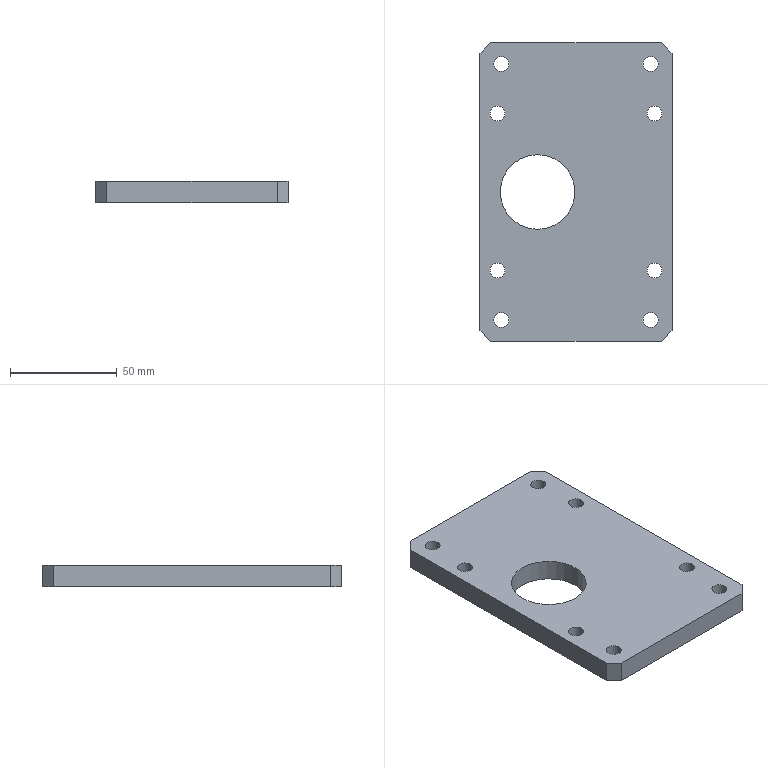Part | NX | features 5003_202_Mounting plate 2 | 1 solid | 19 faces | box 90 x 140 x 10 mm | volume 112800 mm3 | plane 10 | cylinder 9 | commonest cylinder face diameters 7 x8 35 x1
STEP:
#1=CARTESIAN_POINT('',(136.525,-252.,-325.));
#2=VERTEX_POINT('',#1);
#3=CARTESIAN_POINT('',(216.525,-252.,-325.));
#4=VERTEX_POINT('',#3);
#5=CARTESIAN_POINT('',(158.525,-252.,-325.));
#6=DIRECTION('',(1.,0.,0.));
#7=VECTOR('',#6,1000.);
#8=LINE('',#5,#7);
#9=EDGE_CURVE('',#2,#4,#8,.T.);
#10=ORIENTED_EDGE('',*,*,#9,.T.);
#11=CARTESIAN_POINT('',(216.525,-252.,-335.));
#12=VERTEX_POINT('',#11);
#13=CARTESIAN_POINT('',(216.525,-252.,-335.));
#14=DIRECTION('',(0.,0.,-1.));
#15=VECTOR('',#14,1000.);
#16=LINE('',#13,#15);
#17=EDGE_CURVE('',#4,#12,#16,.T.);
#18=ORIENTED_EDGE('',*,*,#17,.T.);
#19=CARTESIAN_POINT('',(136.525,-252.,-335.));
#20=VERTEX_POINT('',#19);
#21=CARTESIAN_POINT('',(158.525,-252.,-335.));
#22=DIRECTION('',(1.,0.,0.));
#23=VECTOR('',#22,1000.);
#24=LINE('',#21,#23);
#25=EDGE_CURVE('',#20,#12,#24,.T.);
#26=ORIENTED_EDGE('',*,*,#25,.F.);
#27=CARTESIAN_POINT('',(136.525,-252.,-325.));
#28=DIRECTION('',(0.,0.,1.));
#29=VECTOR('',#28,1000.);
#30=LINE('',#27,#29);
#31=EDGE_CURVE('',#20,#2,#30,.T.);
#32=ORIENTED_EDGE('',*,*,#31,.T.);
#33=EDGE_LOOP('',(#10,#18,#26,#32));
#34=FACE_BOUND('',#33,.T.);
#35=CARTESIAN_POINT('',(158.525,-252.,-325.));
#36=DIRECTION('',(0.,1.,0.));
#37=DIRECTION('',(0.,0.,-1.));
#38=AXIS2_PLACEMENT_3D('',#35,#36,#37);
#39=PLANE('',#38);
#40=ADVANCED_FACE('',(#34),#39,.T.);
#41=CARTESIAN_POINT('',(131.525,-387.,-325.));
#42=VERTEX_POINT('',#41);
#43=CARTESIAN_POINT('',(131.525,-257.,-325.));
#44=VERTEX_POINT('',#43);
#45=CARTESIAN_POINT('',(131.525,-322.,-325.));
#46=DIRECTION('',(0.,1.,0.));
#47=VECTOR('',#46,1000.);
#48=LINE('',#45,#47);
#49=EDGE_CURVE('',#42,#44,#48,.T.);
#50=ORIENTED_EDGE('',*,*,#49,.T.);
#51=CARTESIAN_POINT('',(131.525,-257.,-335.));
#52=VERTEX_POINT('',#51);
#53=CARTESIAN_POINT('',(131.525,-257.,-325.));
#54=DIRECTION('',(0.,0.,-1.));
#55=VECTOR('',#54,1000.);
#56=LINE('',#53,#55);
#57=EDGE_CURVE('',#44,#52,#56,.T.);
#58=ORIENTED_EDGE('',*,*,#57,.T.);
#59=CARTESIAN_POINT('',(131.525,-387.,-335.));
#60=VERTEX_POINT('',#59);
#61=CARTESIAN_POINT('',(131.525,-322.,-335.));
#62=DIRECTION('',(0.,1.,0.));
#63=VECTOR('',#62,1000.);
#64=LINE('',#61,#63);
#65=EDGE_CURVE('',#60,#52,#64,.T.);
#66=ORIENTED_EDGE('',*,*,#65,.F.);
#67=CARTESIAN_POINT('',(131.525,-387.,-325.));
#68=DIRECTION('',(0.,0.,1.));
#69=VECTOR('',#68,1000.);
#70=LINE('',#67,#69);
#71=EDGE_CURVE('',#60,#42,#70,.T.);
#72=ORIENTED_EDGE('',*,*,#71,.T.);
#73=EDGE_LOOP('',(#50,#58,#66,#72));
#74=FACE_BOUND('',#73,.T.);
#75=CARTESIAN_POINT('',(131.525,-322.,-325.));
#76=DIRECTION('',(-1.,0.,0.));
#77=DIRECTION('',(0.,0.,1.));
#78=AXIS2_PLACEMENT_3D('',#75,#76,#77);
#79=PLANE('',#78);
#80=ADVANCED_FACE('',(#74),#79,.T.);
#81=CARTESIAN_POINT('',(136.525,-392.,-325.));
#82=VERTEX_POINT('',#81);
#83=CARTESIAN_POINT('',(216.525,-392.,-325.));
#84=VERTEX_POINT('',#83);
#85=CARTESIAN_POINT('',(158.525,-392.,-325.));
#86=DIRECTION('',(1.,0.,0.));
#87=VECTOR('',#86,1000.);
#88=LINE('',#85,#87);
#89=EDGE_CURVE('',#82,#84,#88,.T.);
#90=ORIENTED_EDGE('',*,*,#89,.F.);
#91=CARTESIAN_POINT('',(136.525,-392.,-335.));
#92=VERTEX_POINT('',#91);
#93=CARTESIAN_POINT('',(136.525,-392.,-335.));
#94=DIRECTION('',(0.,0.,-1.));
#95=VECTOR('',#94,1000.);
#96=LINE('',#93,#95);
#97=EDGE_CURVE('',#82,#92,#96,.T.);
#98=ORIENTED_EDGE('',*,*,#97,.T.);
#99=CARTESIAN_POINT('',(216.525,-392.,-335.));
#100=VERTEX_POINT('',#99);
#101=CARTESIAN_POINT('',(158.525,-392.,-335.));
#102=DIRECTION('',(1.,0.,0.));
#103=VECTOR('',#102,1000.);
#104=LINE('',#101,#103);
#105=EDGE_CURVE('',#92,#100,#104,.T.);
#106=ORIENTED_EDGE('',*,*,#105,.T.);
#107=CARTESIAN_POINT('',(216.525,-392.,-325.));
#108=DIRECTION('',(0.,0.,1.));
#109=VECTOR('',#108,1000.);
#110=LINE('',#107,#109);
#111=EDGE_CURVE('',#100,#84,#110,.T.);
#112=ORIENTED_EDGE('',*,*,#111,.T.);
#113=EDGE_LOOP('',(#90,#98,#106,#112));
#114=FACE_BOUND('',#113,.T.);
#115=CARTESIAN_POINT('',(158.525,-392.,-325.));
#116=DIRECTION('',(0.,1.,0.));
#117=DIRECTION('',(-1.,0.,0.));
#118=AXIS2_PLACEMENT_3D('',#115,#116,#117);
#119=PLANE('',#118);
#120=ADVANCED_FACE('',(#114),#119,.F.);
#121=CARTESIAN_POINT('',(211.525,-258.5,-325.));
#122=VERTEX_POINT('',#121);
#123=CARTESIAN_POINT('',(211.525,-262.,-325.));
#124=DIRECTION('',(0.,0.,1.));
#125=DIRECTION('',(0.,1.,0.));
#126=AXIS2_PLACEMENT_3D('',#123,#124,#125);
#127=CIRCLE('',#126,3.5);
#128=EDGE_CURVE('',#122,#122,#127,.F.);
#129=ORIENTED_EDGE('',*,*,#128,.F.);
#130=EDGE_LOOP('',(#129));
#131=FACE_BOUND('',#130,.T.);
#132=CARTESIAN_POINT('',(211.525,-258.5,-335.));
#133=VERTEX_POINT('',#132);
#134=CARTESIAN_POINT('',(211.525,-262.,-335.));
#135=DIRECTION('',(0.,0.,1.));
#136=DIRECTION('',(0.,1.,0.));
#137=AXIS2_PLACEMENT_3D('',#134,#135,#136);
#138=CIRCLE('',#137,3.5);
#139=EDGE_CURVE('',#133,#133,#138,.F.);
#140=ORIENTED_EDGE('',*,*,#139,.T.);
#141=EDGE_LOOP('',(#140));
#142=FACE_BOUND('',#141,.T.);
#143=CARTESIAN_POINT('',(211.525,-262.,-325.));
#144=DIRECTION('',(0.,0.,-1.));
#145=DIRECTION('',(0.,-1.,0.));
#146=AXIS2_PLACEMENT_3D('',#143,#144,#145);
#147=CYLINDRICAL_SURFACE('',#146,3.5);
#148=ADVANCED_FACE('',(#131,#142),#147,.F.);
#149=CARTESIAN_POINT('',(158.525,-304.5,-325.));
#150=VERTEX_POINT('',#149);
#151=CARTESIAN_POINT('',(158.525,-322.,-325.));
#152=DIRECTION('',(0.,0.,1.));
#153=DIRECTION('',(0.,1.,0.));
#154=AXIS2_PLACEMENT_3D('',#151,#152,#153);
#155=CIRCLE('',#154,17.5);
#156=EDGE_CURVE('',#150,#150,#155,.T.);
#157=ORIENTED_EDGE('',*,*,#156,.T.);
#158=EDGE_LOOP('',(#157));
#159=FACE_BOUND('',#158,.T.);
#160=CARTESIAN_POINT('',(158.525,-304.5,-335.));
#161=VERTEX_POINT('',#160);
#162=CARTESIAN_POINT('',(158.525,-322.,-335.));
#163=DIRECTION('',(0.,0.,1.));
#164=DIRECTION('',(0.,1.,0.));
#165=AXIS2_PLACEMENT_3D('',#162,#163,#164);
#166=CIRCLE('',#165,17.5);
#167=EDGE_CURVE('',#161,#161,#166,.T.);
#168=ORIENTED_EDGE('',*,*,#167,.F.);
#169=EDGE_LOOP('',(#168));
#170=FACE_BOUND('',#169,.T.);
#171=CARTESIAN_POINT('',(158.525,-322.,-325.));
#172=DIRECTION('',(0.,0.,-1.));
#173=DIRECTION('',(0.,-1.,0.));
#174=AXIS2_PLACEMENT_3D('',#171,#172,#173);
#175=CYLINDRICAL_SURFACE('',#174,17.5);
#176=ADVANCED_FACE('',(#159,#170),#175,.F.);
#177=CARTESIAN_POINT('',(141.525,-378.5,-325.));
#178=VERTEX_POINT('',#177);
#179=CARTESIAN_POINT('',(141.525,-382.,-325.));
#180=DIRECTION('',(0.,0.,1.));
#181=DIRECTION('',(0.,1.,0.));
#182=AXIS2_PLACEMENT_3D('',#179,#180,#181);
#183=CIRCLE('',#182,3.5);
#184=EDGE_CURVE('',#178,#178,#183,.T.);
#185=ORIENTED_EDGE('',*,*,#184,.T.);
#186=EDGE_LOOP('',(#185));
#187=FACE_BOUND('',#186,.T.);
#188=CARTESIAN_POINT('',(141.525,-378.5,-335.));
#189=VERTEX_POINT('',#188);
#190=CARTESIAN_POINT('',(141.525,-382.,-335.));
#191=DIRECTION('',(0.,0.,1.));
#192=DIRECTION('',(0.,1.,0.));
#193=AXIS2_PLACEMENT_3D('',#190,#191,#192);
#194=CIRCLE('',#193,3.5);
#195=EDGE_CURVE('',#189,#189,#194,.T.);
#196=ORIENTED_EDGE('',*,*,#195,.F.);
#197=EDGE_LOOP('',(#196));
#198=FACE_BOUND('',#197,.T.);
#199=CARTESIAN_POINT('',(141.525,-382.,-325.));
#200=DIRECTION('',(0.,0.,-1.));
#201=DIRECTION('',(0.,-1.,0.));
#202=AXIS2_PLACEMENT_3D('',#199,#200,#201);
#203=CYLINDRICAL_SURFACE('',#202,3.5);
#204=ADVANCED_FACE('',(#187,#198),#203,.F.);
#205=CARTESIAN_POINT('',(139.745,-355.28,-325.));
#206=VERTEX_POINT('',#205);
#207=CARTESIAN_POINT('',(139.745,-358.78,-325.));
#208=DIRECTION('',(0.,0.,1.));
#209=DIRECTION('',(0.,1.,0.));
#210=AXIS2_PLACEMENT_3D('',#207,#208,#209);
#211=CIRCLE('',#210,3.5);
#212=EDGE_CURVE('',#206,#206,#211,.T.);
#213=ORIENTED_EDGE('',*,*,#212,.T.);
#214=EDGE_LOOP('',(#213));
#215=FACE_BOUND('',#214,.T.);
#216=CARTESIAN_POINT('',(139.745,-355.28,-335.));
#217=VERTEX_POINT('',#216);
#218=CARTESIAN_POINT('',(139.745,-358.78,-335.));
#219=DIRECTION('',(0.,0.,1.));
#220=DIRECTION('',(0.,1.,0.));
#221=AXIS2_PLACEMENT_3D('',#218,#219,#220);
#222=CIRCLE('',#221,3.5);
#223=EDGE_CURVE('',#217,#217,#222,.T.);
#224=ORIENTED_EDGE('',*,*,#223,.F.);
#225=EDGE_LOOP('',(#224));
#226=FACE_BOUND('',#225,.T.);
#227=CARTESIAN_POINT('',(139.745,-358.78,-325.));
#228=DIRECTION('',(0.,0.,-1.));
#229=DIRECTION('',(0.,-1.,0.));
#230=AXIS2_PLACEMENT_3D('',#227,#228,#229);
#231=CYLINDRICAL_SURFACE('',#230,3.5);
#232=ADVANCED_FACE('',(#215,#226),#231,.F.);
#233=CARTESIAN_POINT('',(211.525,-378.5,-325.));
#234=VERTEX_POINT('',#233);
#235=CARTESIAN_POINT('',(211.525,-382.,-325.));
#236=DIRECTION('',(0.,0.,1.));
#237=DIRECTION('',(0.,1.,0.));
#238=AXIS2_PLACEMENT_3D('',#235,#236,#237);
#239=CIRCLE('',#238,3.5);
#240=EDGE_CURVE('',#234,#234,#239,.T.);
#241=ORIENTED_EDGE('',*,*,#240,.T.);
#242=EDGE_LOOP('',(#241));
#243=FACE_BOUND('',#242,.T.);
#244=CARTESIAN_POINT('',(211.525,-378.5,-335.));
#245=VERTEX_POINT('',#244);
#246=CARTESIAN_POINT('',(211.525,-382.,-335.));
#247=DIRECTION('',(0.,0.,1.));
#248=DIRECTION('',(0.,1.,0.));
#249=AXIS2_PLACEMENT_3D('',#246,#247,#248);
#250=CIRCLE('',#249,3.5);
#251=EDGE_CURVE('',#245,#245,#250,.T.);
#252=ORIENTED_EDGE('',*,*,#251,.F.);
#253=EDGE_LOOP('',(#252));
#254=FACE_BOUND('',#253,.T.);
#255=CARTESIAN_POINT('',(211.525,-382.,-325.));
#256=DIRECTION('',(0.,0.,-1.));
#257=DIRECTION('',(0.,-1.,0.));
#258=AXIS2_PLACEMENT_3D('',#255,#256,#257);
#259=CYLINDRICAL_SURFACE('',#258,3.5);
#260=ADVANCED_FACE('',(#243,#254),#259,.F.);
#261=CARTESIAN_POINT('',(213.305,-355.28,-325.));
#262=VERTEX_POINT('',#261);
#263=CARTESIAN_POINT('',(213.305,-358.78,-325.));
#264=DIRECTION('',(0.,0.,1.));
#265=DIRECTION('',(0.,1.,0.));
#266=AXIS2_PLACEMENT_3D('',#263,#264,#265);
#267=CIRCLE('',#266,3.5);
#268=EDGE_CURVE('',#262,#262,#267,.T.);
#269=ORIENTED_EDGE('',*,*,#268,.T.);
#270=EDGE_LOOP('',(#269));
#271=FACE_BOUND('',#270,.T.);
#272=CARTESIAN_POINT('',(213.305,-355.28,-335.));
#273=VERTEX_POINT('',#272);
#274=CARTESIAN_POINT('',(213.305,-358.78,-335.));
#275=DIRECTION('',(0.,0.,1.));
#276=DIRECTION('',(0.,1.,0.));
#277=AXIS2_PLACEMENT_3D('',#274,#275,#276);
#278=CIRCLE('',#277,3.5);
#279=EDGE_CURVE('',#273,#273,#278,.T.);
#280=ORIENTED_EDGE('',*,*,#279,.F.);
#281=EDGE_LOOP('',(#280));
#282=FACE_BOUND('',#281,.T.);
#283=CARTESIAN_POINT('',(213.305,-358.78,-325.));
#284=DIRECTION('',(0.,0.,-1.));
#285=DIRECTION('',(0.,-1.,0.));
#286=AXIS2_PLACEMENT_3D('',#283,#284,#285);
#287=CYLINDRICAL_SURFACE('',#286,3.5);
#288=ADVANCED_FACE('',(#271,#282),#287,.F.);
#289=CARTESIAN_POINT('',(213.305,-281.72,-325.));
#290=VERTEX_POINT('',#289);
#291=CARTESIAN_POINT('',(213.305,-285.22,-325.));
#292=DIRECTION('',(0.,0.,1.));
#293=DIRECTION('',(0.,1.,0.));
#294=AXIS2_PLACEMENT_3D('',#291,#292,#293);
#295=CIRCLE('',#294,3.5);
#296=EDGE_CURVE('',#290,#290,#295,.F.);
#297=ORIENTED_EDGE('',*,*,#296,.F.);
#298=EDGE_LOOP('',(#297));
#299=FACE_BOUND('',#298,.T.);
#300=CARTESIAN_POINT('',(213.305,-281.72,-335.));
#301=VERTEX_POINT('',#300);
#302=CARTESIAN_POINT('',(213.305,-285.22,-335.));
#303=DIRECTION('',(0.,0.,1.));
#304=DIRECTION('',(0.,1.,0.));
#305=AXIS2_PLACEMENT_3D('',#302,#303,#304);
#306=CIRCLE('',#305,3.5);
#307=EDGE_CURVE('',#301,#301,#306,.F.);
#308=ORIENTED_EDGE('',*,*,#307,.T.);
#309=EDGE_LOOP('',(#308));
#310=FACE_BOUND('',#309,.T.);
#311=CARTESIAN_POINT('',(213.305,-285.22,-325.));
#312=DIRECTION('',(0.,0.,-1.));
#313=DIRECTION('',(0.,-1.,0.));
#314=AXIS2_PLACEMENT_3D('',#311,#312,#313);
#315=CYLINDRICAL_SURFACE('',#314,3.5);
#316=ADVANCED_FACE('',(#299,#310),#315,.F.);
#317=CARTESIAN_POINT('',(139.745,-281.72,-325.));
#318=VERTEX_POINT('',#317);
#319=CARTESIAN_POINT('',(139.745,-285.22,-325.));
#320=DIRECTION('',(0.,0.,1.));
#321=DIRECTION('',(0.,1.,0.));
#322=AXIS2_PLACEMENT_3D('',#319,#320,#321);
#323=CIRCLE('',#322,3.5);
#324=EDGE_CURVE('',#318,#318,#323,.F.);
#325=ORIENTED_EDGE('',*,*,#324,.F.);
#326=EDGE_LOOP('',(#325));
#327=FACE_BOUND('',#326,.T.);
#328=CARTESIAN_POINT('',(139.745,-281.72,-335.));
#329=VERTEX_POINT('',#328);
#330=CARTESIAN_POINT('',(139.745,-285.22,-335.));
#331=DIRECTION('',(0.,0.,1.));
#332=DIRECTION('',(0.,1.,0.));
#333=AXIS2_PLACEMENT_3D('',#330,#331,#332);
#334=CIRCLE('',#333,3.5);
#335=EDGE_CURVE('',#329,#329,#334,.F.);
#336=ORIENTED_EDGE('',*,*,#335,.T.);
#337=EDGE_LOOP('',(#336));
#338=FACE_BOUND('',#337,.T.);
#339=CARTESIAN_POINT('',(139.745,-285.22,-325.));
#340=DIRECTION('',(0.,0.,-1.));
#341=DIRECTION('',(0.,-1.,0.));
#342=AXIS2_PLACEMENT_3D('',#339,#340,#341);
#343=CYLINDRICAL_SURFACE('',#342,3.5);
#344=ADVANCED_FACE('',(#327,#338),#343,.F.);
#345=CARTESIAN_POINT('',(221.525,-387.,-335.));
#346=VERTEX_POINT('',#345);
#347=CARTESIAN_POINT('',(221.525,-257.,-335.));
#348=VERTEX_POINT('',#347);
#349=CARTESIAN_POINT('',(221.525,-322.,-335.));
#350=DIRECTION('',(0.,1.,0.));
#351=VECTOR('',#350,1000.);
#352=LINE('',#349,#351);
#353=EDGE_CURVE('',#346,#348,#352,.T.);
#354=ORIENTED_EDGE('',*,*,#353,.T.);
#355=CARTESIAN_POINT('',(221.525,-257.,-325.));
#356=VERTEX_POINT('',#355);
#357=CARTESIAN_POINT('',(221.525,-257.,-325.));
#358=DIRECTION('',(0.,0.,1.));
#359=VECTOR('',#358,1000.);
#360=LINE('',#357,#359);
#361=EDGE_CURVE('',#348,#356,#360,.T.);
#362=ORIENTED_EDGE('',*,*,#361,.T.);
#363=CARTESIAN_POINT('',(221.525,-387.,-325.));
#364=VERTEX_POINT('',#363);
#365=CARTESIAN_POINT('',(221.525,-322.,-325.));
#366=DIRECTION('',(0.,1.,0.));
#367=VECTOR('',#366,1000.);
#368=LINE('',#365,#367);
#369=EDGE_CURVE('',#364,#356,#368,.T.);
#370=ORIENTED_EDGE('',*,*,#369,.F.);
#371=CARTESIAN_POINT('',(221.525,-387.,-325.));
#372=DIRECTION('',(0.,0.,-1.));
#373=VECTOR('',#372,1000.);
#374=LINE('',#371,#373);
#375=EDGE_CURVE('',#364,#346,#374,.T.);
#376=ORIENTED_EDGE('',*,*,#375,.T.);
#377=EDGE_LOOP('',(#354,#362,#370,#376));
#378=FACE_BOUND('',#377,.T.);
#379=CARTESIAN_POINT('',(221.525,-322.,-325.));
#380=DIRECTION('',(-1.,0.,0.));
#381=DIRECTION('',(0.,0.,1.));
#382=AXIS2_PLACEMENT_3D('',#379,#380,#381);
#383=PLANE('',#382);
#384=ADVANCED_FACE('',(#378),#383,.F.);
#385=CARTESIAN_POINT('',(141.525,-258.5,-325.));
#386=VERTEX_POINT('',#385);
#387=CARTESIAN_POINT('',(141.525,-262.,-325.));
#388=DIRECTION('',(0.,0.,1.));
#389=DIRECTION('',(0.,1.,0.));
#390=AXIS2_PLACEMENT_3D('',#387,#388,#389);
#391=CIRCLE('',#390,3.5);
#392=EDGE_CURVE('',#386,#386,#391,.F.);
#393=ORIENTED_EDGE('',*,*,#392,.F.);
#394=EDGE_LOOP('',(#393));
#395=FACE_BOUND('',#394,.T.);
#396=CARTESIAN_POINT('',(141.525,-258.5,-335.));
#397=VERTEX_POINT('',#396);
#398=CARTESIAN_POINT('',(141.525,-262.,-335.));
#399=DIRECTION('',(0.,0.,1.));
#400=DIRECTION('',(0.,1.,0.));
#401=AXIS2_PLACEMENT_3D('',#398,#399,#400);
#402=CIRCLE('',#401,3.5);
#403=EDGE_CURVE('',#397,#397,#402,.F.);
#404=ORIENTED_EDGE('',*,*,#403,.T.);
#405=EDGE_LOOP('',(#404));
#406=FACE_BOUND('',#405,.T.);
#407=CARTESIAN_POINT('',(141.525,-262.,-325.));
#408=DIRECTION('',(0.,0.,-1.));
#409=DIRECTION('',(0.,-1.,0.));
#410=AXIS2_PLACEMENT_3D('',#407,#408,#409);
#411=CYLINDRICAL_SURFACE('',#410,3.5);
#412=ADVANCED_FACE('',(#395,#406),#411,.F.);
#413=ORIENTED_EDGE('',*,*,#369,.T.);
#414=CARTESIAN_POINT('',(222.525,-258.,-325.));
#415=DIRECTION('',(-0.7071,0.7071,0.));
#416=VECTOR('',#415,1000.);
#417=LINE('',#414,#416);
#418=EDGE_CURVE('',#356,#4,#417,.T.);
#419=ORIENTED_EDGE('',*,*,#418,.T.);
#420=ORIENTED_EDGE('',*,*,#9,.F.);
#421=CARTESIAN_POINT('',(112.525,-276.,-325.));
#422=DIRECTION('',(0.7071,0.7071,0.));
#423=VECTOR('',#422,1000.);
#424=LINE('',#421,#423);
#425=EDGE_CURVE('',#2,#44,#424,.F.);
#426=ORIENTED_EDGE('',*,*,#425,.T.);
#427=ORIENTED_EDGE('',*,*,#49,.F.);
#428=CARTESIAN_POINT('',(112.525,-368.,-325.));
#429=DIRECTION('',(0.7071,-0.7071,0.));
#430=VECTOR('',#429,1000.);
#431=LINE('',#428,#430);
#432=EDGE_CURVE('',#42,#82,#431,.T.);
#433=ORIENTED_EDGE('',*,*,#432,.T.);
#434=ORIENTED_EDGE('',*,*,#89,.T.);
#435=CARTESIAN_POINT('',(222.525,-386.,-325.));
#436=DIRECTION('',(-0.7071,-0.7071,0.));
#437=VECTOR('',#436,1000.);
#438=LINE('',#435,#437);
#439=EDGE_CURVE('',#84,#364,#438,.F.);
#440=ORIENTED_EDGE('',*,*,#439,.T.);
#441=EDGE_LOOP('',(#413,#419,#420,#426,#427,#433,#434,#440));
#442=FACE_BOUND('',#441,.T.);
#443=ORIENTED_EDGE('',*,*,#324,.T.);
#444=EDGE_LOOP('',(#443));
#445=FACE_BOUND('',#444,.T.);
#446=ORIENTED_EDGE('',*,*,#296,.T.);
#447=EDGE_LOOP('',(#446));
#448=FACE_BOUND('',#447,.T.);
#449=ORIENTED_EDGE('',*,*,#268,.F.);
#450=EDGE_LOOP('',(#449));
#451=FACE_BOUND('',#450,.T.);
#452=ORIENTED_EDGE('',*,*,#240,.F.);
#453=EDGE_LOOP('',(#452));
#454=FACE_BOUND('',#453,.T.);
#455=ORIENTED_EDGE('',*,*,#212,.F.);
#456=EDGE_LOOP('',(#455));
#457=FACE_BOUND('',#456,.T.);
#458=ORIENTED_EDGE('',*,*,#184,.F.);
#459=EDGE_LOOP('',(#458));
#460=FACE_BOUND('',#459,.T.);
#461=ORIENTED_EDGE('',*,*,#156,.F.);
#462=EDGE_LOOP('',(#461));
#463=FACE_BOUND('',#462,.T.);
#464=ORIENTED_EDGE('',*,*,#128,.T.);
#465=EDGE_LOOP('',(#464));
#466=FACE_BOUND('',#465,.T.);
#467=ORIENTED_EDGE('',*,*,#392,.T.);
#468=EDGE_LOOP('',(#467));
#469=FACE_BOUND('',#468,.T.);
#470=CARTESIAN_POINT('',(158.525,-322.,-325.));
#471=DIRECTION('',(0.,0.,1.));
#472=DIRECTION('',(0.,1.,0.));
#473=AXIS2_PLACEMENT_3D('',#470,#471,#472);
#474=PLANE('',#473);
#475=ADVANCED_FACE('',(#442,#445,#448,#451,#454,#457,#460,#463,#466,#469),#474,.T.);
#476=ORIENTED_EDGE('',*,*,#25,.T.);
#477=CARTESIAN_POINT('',(216.525,-252.,-335.));
#478=DIRECTION('',(0.7071,-0.7071,0.));
#479=VECTOR('',#478,1000.);
#480=LINE('',#477,#479);
#481=EDGE_CURVE('',#12,#348,#480,.T.);
#482=ORIENTED_EDGE('',*,*,#481,.T.);
#483=ORIENTED_EDGE('',*,*,#353,.F.);
#484=CARTESIAN_POINT('',(221.525,-387.,-335.));
#485=DIRECTION('',(0.7071,0.7071,0.));
#486=VECTOR('',#485,1000.);
#487=LINE('',#484,#486);
#488=EDGE_CURVE('',#346,#100,#487,.F.);
#489=ORIENTED_EDGE('',*,*,#488,.T.);
#490=ORIENTED_EDGE('',*,*,#105,.F.);
#491=CARTESIAN_POINT('',(136.525,-392.,-335.));
#492=DIRECTION('',(-0.7071,0.7071,0.));
#493=VECTOR('',#492,1000.);
#494=LINE('',#491,#493);
#495=EDGE_CURVE('',#92,#60,#494,.T.);
#496=ORIENTED_EDGE('',*,*,#495,.T.);
#497=ORIENTED_EDGE('',*,*,#65,.T.);
#498=CARTESIAN_POINT('',(131.525,-257.,-335.));
#499=DIRECTION('',(-0.7071,-0.7071,0.));
#500=VECTOR('',#499,1000.);
#501=LINE('',#498,#500);
#502=EDGE_CURVE('',#52,#20,#501,.F.);
#503=ORIENTED_EDGE('',*,*,#502,.T.);
#504=EDGE_LOOP('',(#476,#482,#483,#489,#490,#496,#497,#503));
#505=FACE_BOUND('',#504,.T.);
#506=ORIENTED_EDGE('',*,*,#335,.F.);
#507=EDGE_LOOP('',(#506));
#508=FACE_BOUND('',#507,.T.);
#509=ORIENTED_EDGE('',*,*,#307,.F.);
#510=EDGE_LOOP('',(#509));
#511=FACE_BOUND('',#510,.T.);
#512=ORIENTED_EDGE('',*,*,#279,.T.);
#513=EDGE_LOOP('',(#512));
#514=FACE_BOUND('',#513,.T.);
#515=ORIENTED_EDGE('',*,*,#251,.T.);
#516=EDGE_LOOP('',(#515));
#517=FACE_BOUND('',#516,.T.);
#518=ORIENTED_EDGE('',*,*,#223,.T.);
#519=EDGE_LOOP('',(#518));
#520=FACE_BOUND('',#519,.T.);
#521=ORIENTED_EDGE('',*,*,#195,.T.);
#522=EDGE_LOOP('',(#521));
#523=FACE_BOUND('',#522,.T.);
#524=ORIENTED_EDGE('',*,*,#167,.T.);
#525=EDGE_LOOP('',(#524));
#526=FACE_BOUND('',#525,.T.);
#527=ORIENTED_EDGE('',*,*,#139,.F.);
#528=EDGE_LOOP('',(#527));
#529=FACE_BOUND('',#528,.T.);
#530=ORIENTED_EDGE('',*,*,#403,.F.);
#531=EDGE_LOOP('',(#530));
#532=FACE_BOUND('',#531,.T.);
#533=CARTESIAN_POINT('',(158.525,-322.,-335.));
#534=DIRECTION('',(0.,0.,1.));
#535=DIRECTION('',(0.,1.,0.));
#536=AXIS2_PLACEMENT_3D('',#533,#534,#535);
#537=PLANE('',#536);
#538=ADVANCED_FACE('',(#505,#508,#511,#514,#517,#520,#523,#526,#529,#532),#537,.F.);
#539=ORIENTED_EDGE('',*,*,#418,.F.);
#540=ORIENTED_EDGE('',*,*,#361,.F.);
#541=ORIENTED_EDGE('',*,*,#481,.F.);
#542=ORIENTED_EDGE('',*,*,#17,.F.);
#543=EDGE_LOOP('',(#539,#540,#541,#542));
#544=FACE_BOUND('',#543,.T.);
#545=CARTESIAN_POINT('',(216.525,-252.,-325.));
#546=DIRECTION('',(0.7071,0.7071,0.));
#547=DIRECTION('',(0.,0.,1.));
#548=AXIS2_PLACEMENT_3D('',#545,#546,#547);
#549=PLANE('',#548);
#550=ADVANCED_FACE('',(#544),#549,.T.);
#551=ORIENTED_EDGE('',*,*,#425,.F.);
#552=ORIENTED_EDGE('',*,*,#31,.F.);
#553=ORIENTED_EDGE('',*,*,#502,.F.);
#554=ORIENTED_EDGE('',*,*,#57,.F.);
#555=EDGE_LOOP('',(#551,#552,#553,#554));
#556=FACE_BOUND('',#555,.T.);
#557=CARTESIAN_POINT('',(131.525,-257.,-325.));
#558=DIRECTION('',(0.7071,-0.7071,0.));
#559=DIRECTION('',(0.,0.,-1.));
#560=AXIS2_PLACEMENT_3D('',#557,#558,#559);
#561=PLANE('',#560);
#562=ADVANCED_FACE('',(#556),#561,.F.);
#563=ORIENTED_EDGE('',*,*,#432,.F.);
#564=ORIENTED_EDGE('',*,*,#71,.F.);
#565=ORIENTED_EDGE('',*,*,#495,.F.);
#566=ORIENTED_EDGE('',*,*,#97,.F.);
#567=EDGE_LOOP('',(#563,#564,#565,#566));
#568=FACE_BOUND('',#567,.T.);
#569=CARTESIAN_POINT('',(136.525,-392.,-325.));
#570=DIRECTION('',(-0.7071,-0.7071,0.));
#571=DIRECTION('',(0.,0.,1.));
#572=AXIS2_PLACEMENT_3D('',#569,#570,#571);
#573=PLANE('',#572);
#574=ADVANCED_FACE('',(#568),#573,.T.);
#575=ORIENTED_EDGE('',*,*,#439,.F.);
#576=ORIENTED_EDGE('',*,*,#111,.F.);
#577=ORIENTED_EDGE('',*,*,#488,.F.);
#578=ORIENTED_EDGE('',*,*,#375,.F.);
#579=EDGE_LOOP('',(#575,#576,#577,#578));
#580=FACE_BOUND('',#579,.T.);
#581=CARTESIAN_POINT('',(221.525,-387.,-325.));
#582=DIRECTION('',(-0.7071,0.7071,0.));
#583=DIRECTION('',(0.,0.,-1.));
#584=AXIS2_PLACEMENT_3D('',#581,#582,#583);
#585=PLANE('',#584);
#586=ADVANCED_FACE('',(#580),#585,.F.);
#587=CLOSED_SHELL('',(#40,#80,#120,#148,#176,#204,#232,#260,#288,#316,#344,#384,#412,#475,#538,#550,#562,#574,#586));
#588=MANIFOLD_SOLID_BREP('',#587);
#589=(LENGTH_UNIT()NAMED_UNIT(*)SI_UNIT(.MILLI.,.METRE.));
#590=UNCERTAINTY_MEASURE_WITH_UNIT(LENGTH_MEASURE(0.00001),#589,'','');
#591=(NAMED_UNIT(*)PLANE_ANGLE_UNIT()SI_UNIT($,.RADIAN.));
#592=(NAMED_UNIT(*)SI_UNIT($,.STERADIAN.)SOLID_ANGLE_UNIT());
#593=(GEOMETRIC_REPRESENTATION_CONTEXT(3)GLOBAL_UNCERTAINTY_ASSIGNED_CONTEXT((#590))GLOBAL_UNIT_ASSIGNED_CONTEXT((#589,#591,#592))REPRESENTATION_CONTEXT('',''));
#594=ADVANCED_BREP_SHAPE_REPRESENTATION('',(#588),#593);